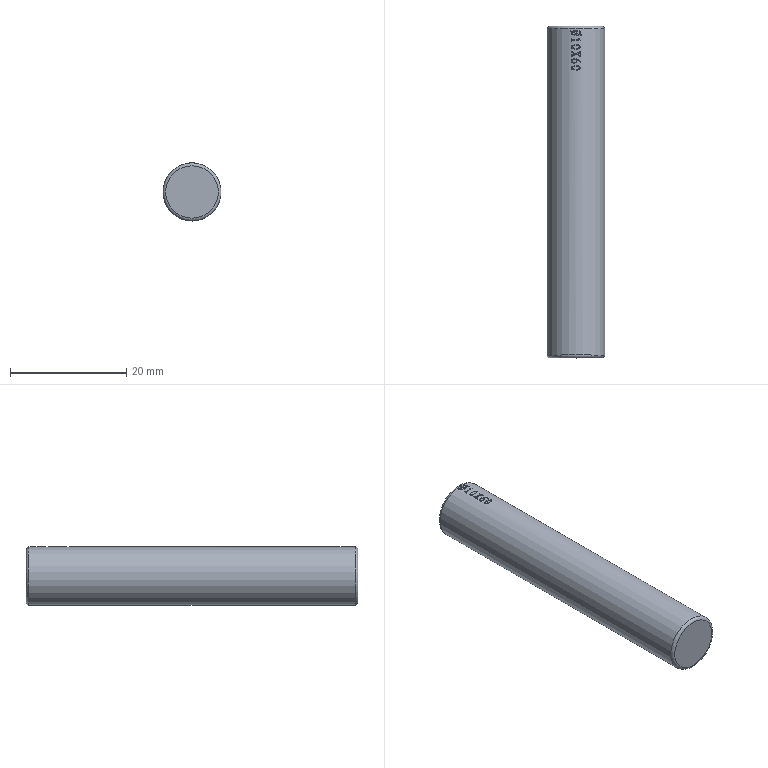Part | STEP file | solid 60 | 1 solid | 77 faces | box 10 x 57 x 10 mm | volume 4325 mm3 | plane 38 | other 29 | cylinder 7 | torus 2 | cone 1 | commonest cylinder face diameters 10 x6 5 x1